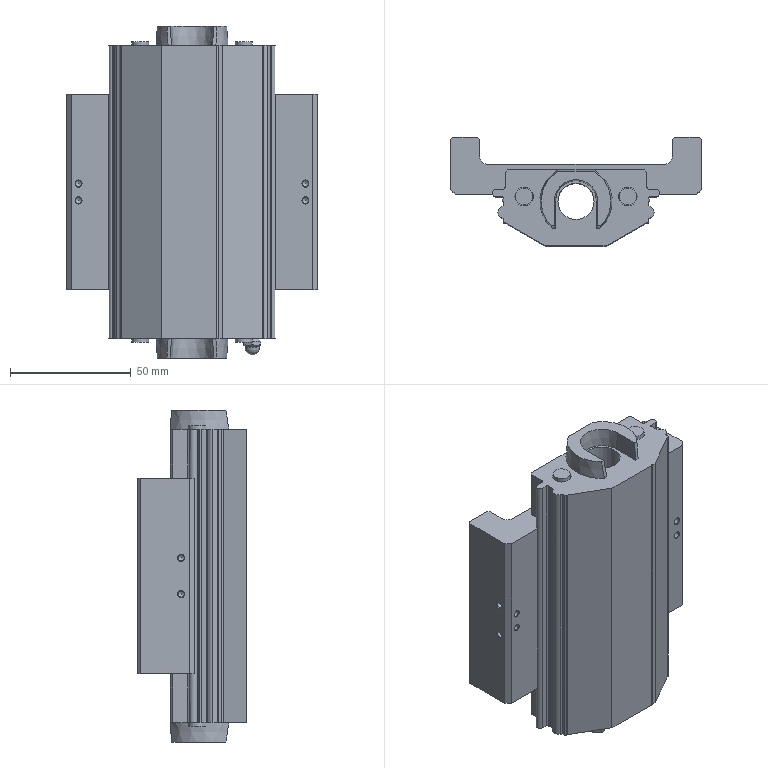Part | STEP file | LX4520CP-MX-B1-590-EP3-ASL_bl | 1 solid | 160 faces | box 104 x 45 x 137.6 mm | volume 272574 mm3 | plane 83 | cylinder 44 | cone 32 | sphere 1 | commonest cylinder face diameters 2.459 x8 2 x6 1.6 x4 4.917 x4 5.2 x4 7 x4